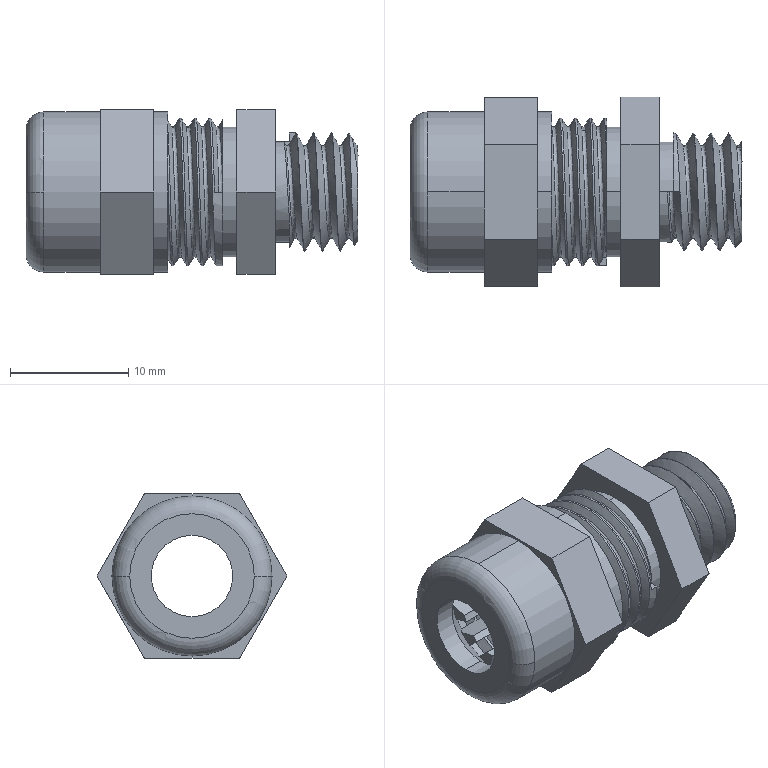Part | SolidWorks | features BaseBody 1 | 1 solid | 239 faces | box 28.1 x 16.062 x 13.91 mm | volume 2026 mm3 | cylinder 143 | plane 74 | cone 12 | spline 8 | torus 2 | commonest cylinder face diameters 11 x113 12.5 x11 10 x7 6.9 x4 7.5 x2 8.5 x2